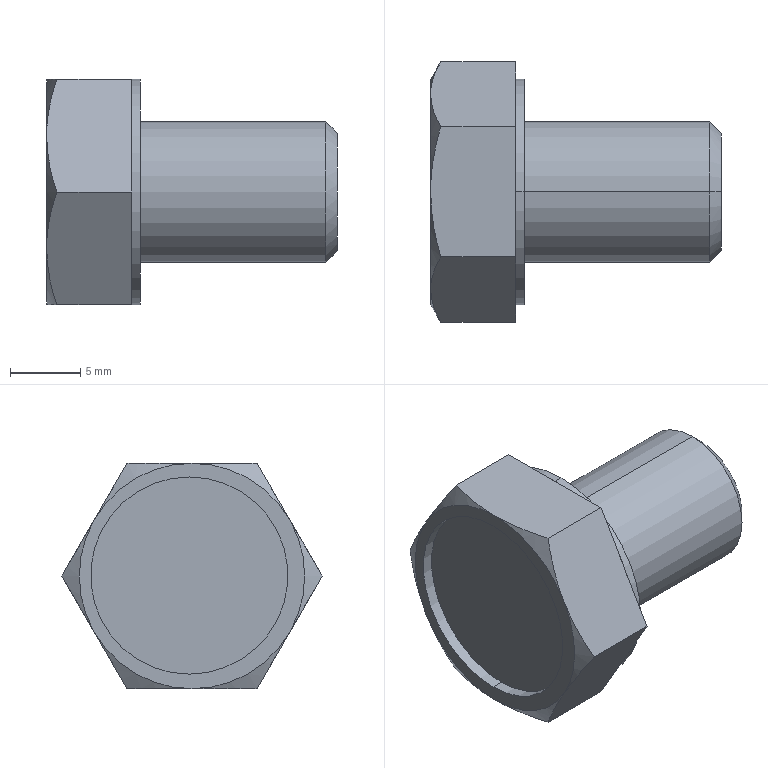Part | STEP file | formed hex screw_am_B18.2.3.2M - Formed hex screw, M10 x 1.5 x 14 --14WN | 1 solid | 30 faces | box 20.63 x 18.475 x 16 mm | volume 2415 mm3 | plane 16 | cone 8 | cylinder 6 | commonest cylinder face diameters 10 x2 14 x2 16 x2